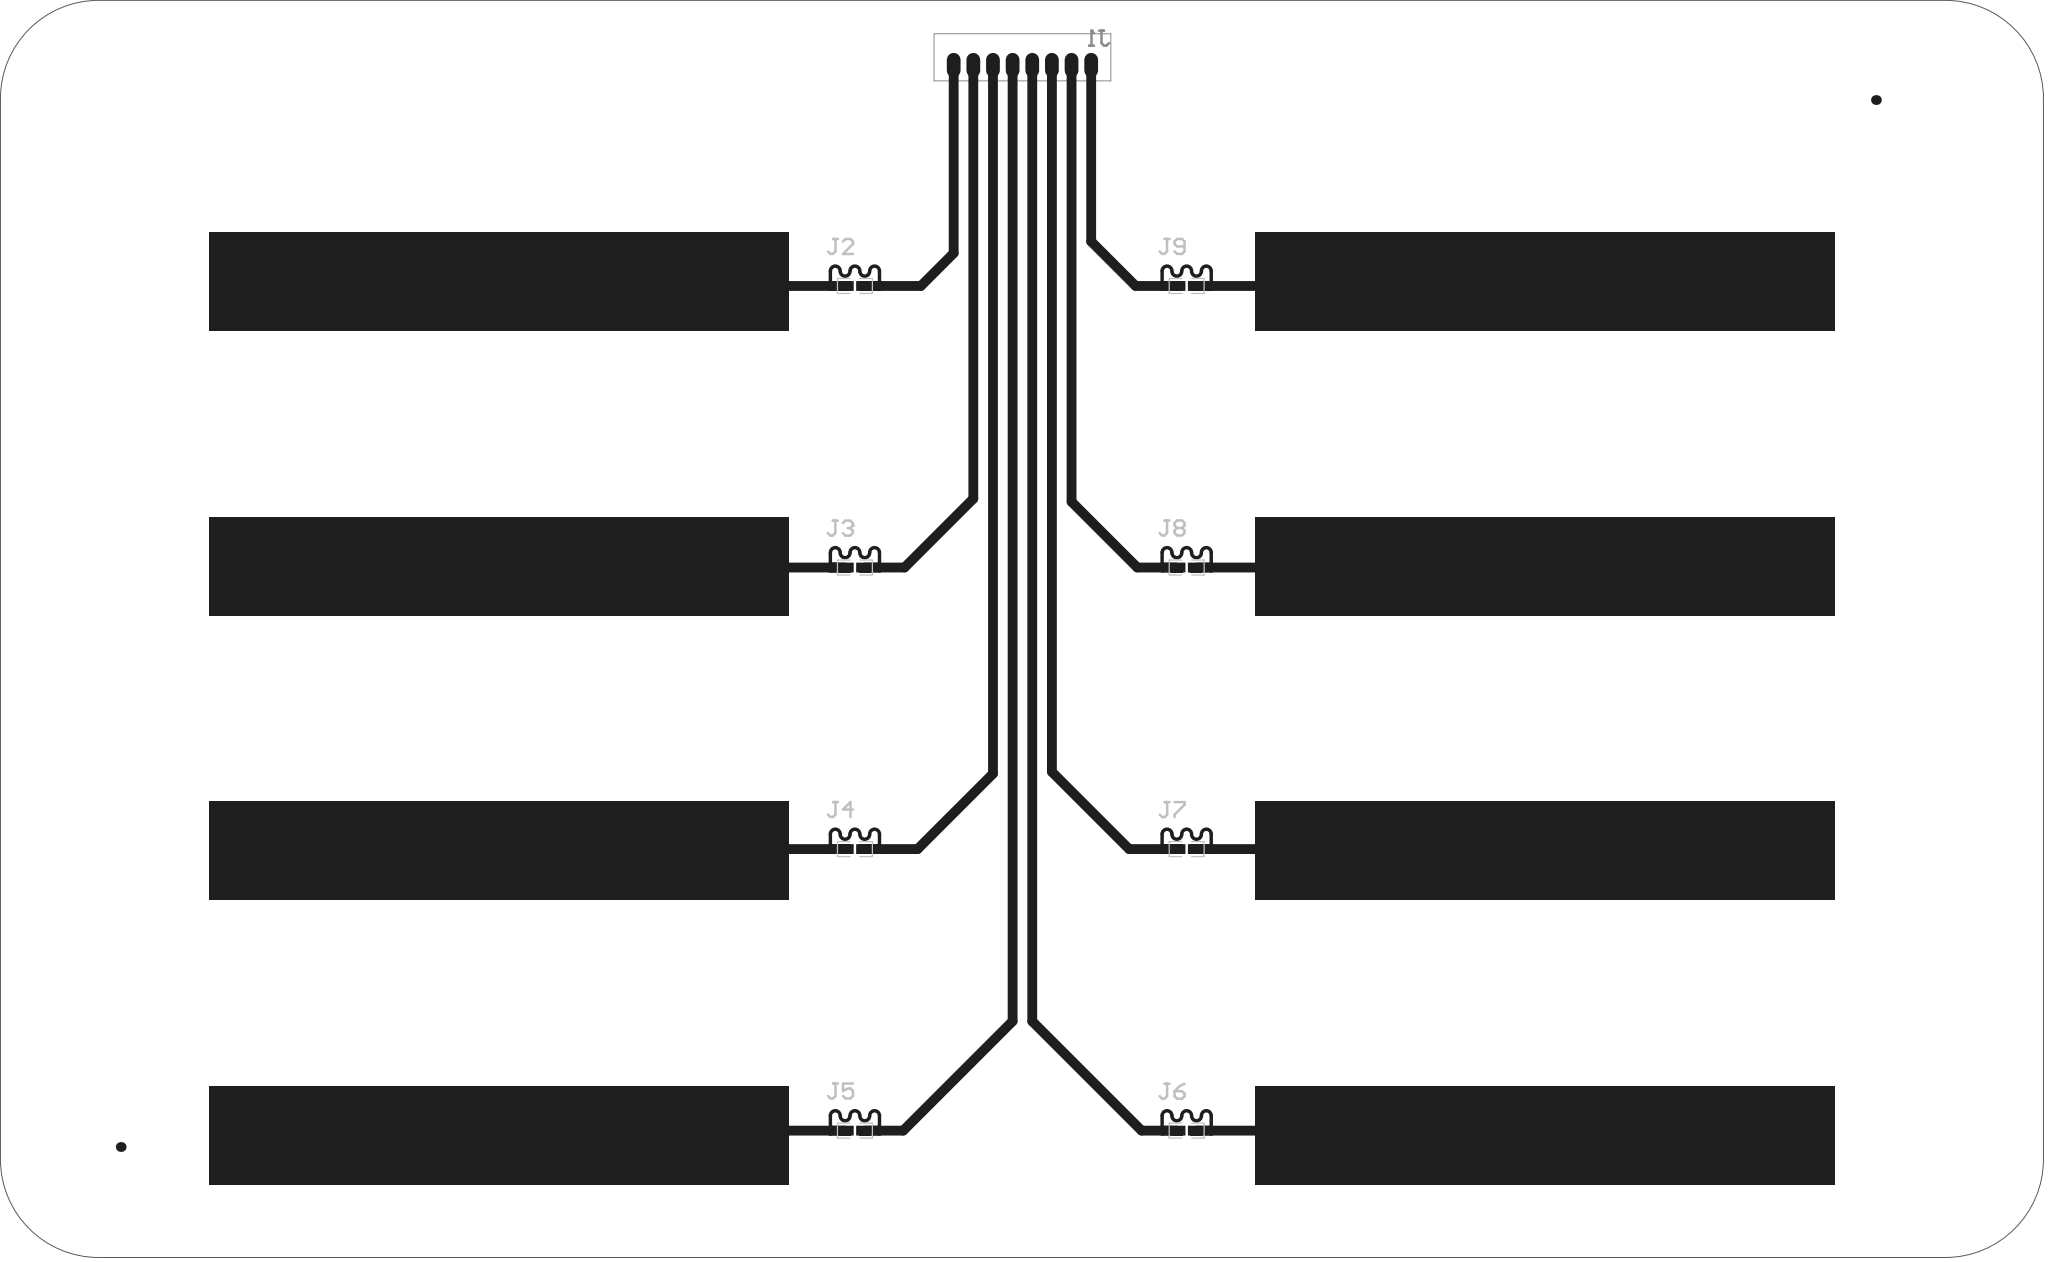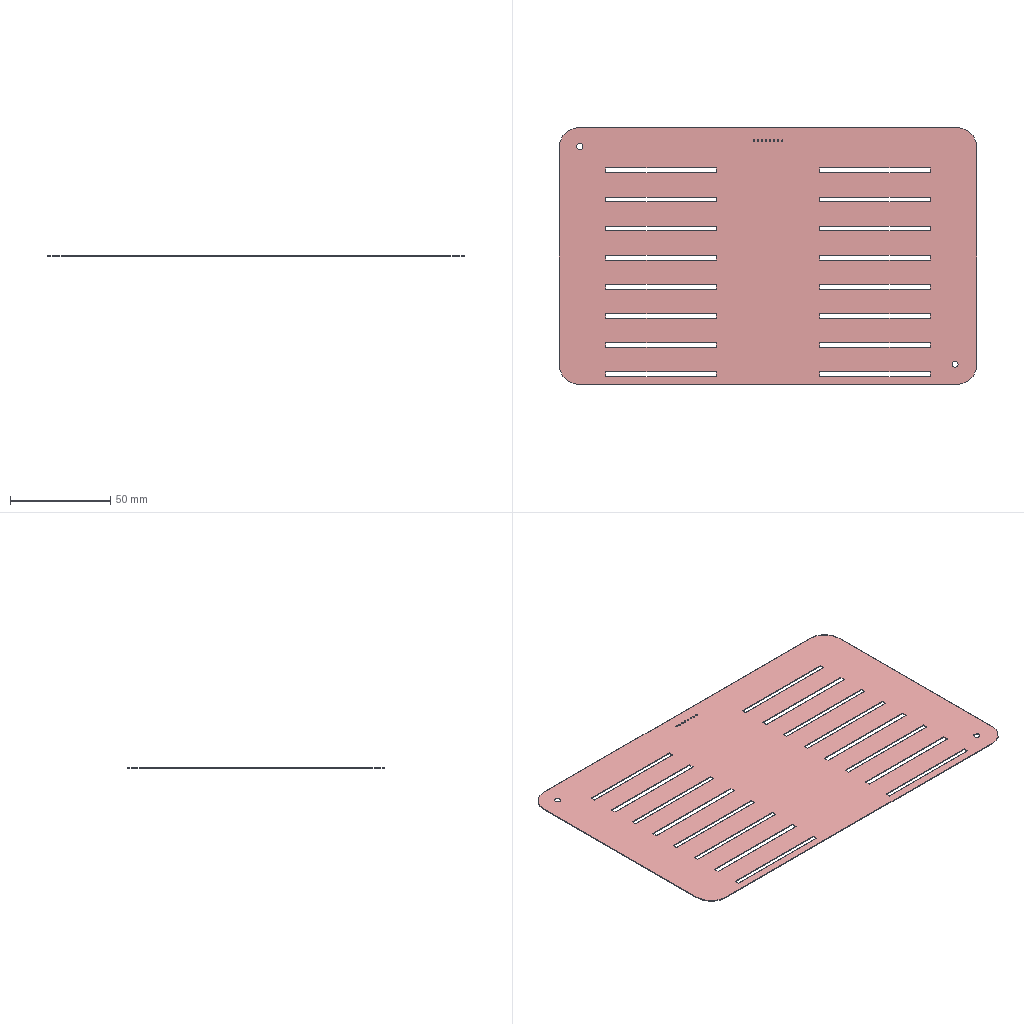Circuit board layout | Altium Designer | box 208 x 128 x 0.4 mm
Layer stack:
# Altium Designer layer stack of  (unit mm; dielectric type: 0 none, 1 core, 2 prepreg, 3 surface material)
index,name,kind,layer,copper_thickness_mm,dielectric_type,dielectric_thickness_mm,dielectric_material,dielectric_constant
0,Top Paste,other,,,,,,
1,Top Overlay,other,,,,,,
2,Top Solder,dielectric,,,3,0.0102,Solder Resist,3.5
3,Top Layer,copper,Top Layer,0.0356,,,,
4,Dielectric 1,dielectric,,,0,0.32,FR-4,4.8
5,Bottom Layer,copper,Bottom Layer,0.0356,,,,
6,Bottom Solder,dielectric,,,3,0.0102,Solder Resist,3.5
7,Bottom Overlay,other,,,,,,
8,Bottom Paste,other,,,,,,
# drill layer pairs: low layer,high layer
drill_pair,Top Layer,Bottom Layer
Part placement:
Designator,Comment,Layer,Footprint,Center-X(mm),Center-Y(mm),Rotation
B15,Pth,TopLayer,55*10*1MM,147.25,89.4,180
B13,Pth,TopLayer,55*10*1MM,147.25,60.4,180
B11,Pth,TopLayer,55*10*1MM,147.25,31.4,180
B9,Pth,TopLayer,55*10*1MM,147.25,2.4,180
B5,Pth,TopLayer,55*10*1MM,40.75,31.4,180
B3,Pth,TopLayer,55*10*1MM,40.75,60.4,180
B1,Pth,TopLayer,55*10*1MM,40.75,89.4,180
B7,Pth,TopLayer,55*10*1MM,40.75,2.4,180
J9,FPC,TopLayer,异形电阻,110.771,88.917,90
J3,FPC,TopLayer,异形电阻,76.996,60.251,90
J7,FPC,TopLayer,异形电阻,110.771,31.584,90
J5,FPC,TopLayer,异形电阻,76.996,2.917,90
J8,FPC,TopLayer,异形电阻,110.771,60.251,90
J6,FPC,TopLayer,异形电阻,110.771,2.917,90
J4,FPC,TopLayer,异形电阻,76.996,31.584,90
J2,FPC,TopLayer,异形电阻,76.996,88.917,90
J1,HX-2.0mm-8P THT connector with latch,BottomLayer,HX2.0-8P,94.05,111.4,0
Pad and via stacks:
# Altium Designer via and pad stacks of  (unit mm). Each distinct definition once, with the count of objects using it.
# via: kind,start_layer,end_layer,hole_mm,diameter_mm,mode(0 simple;1 top-mid-bottom;2 full stack),diameter_per_layer,count,example_net
# pad: kind,layer,hole_mm,hole_type(0 round;1 square;2 slot),plating,top_size,top_shape(1 round;2 rect;3 octagon;9 rounded rect),mid_size,bottom_size,mode,footprint,size_per_layer,count,example
pad,Top Layer,0,0,plated,1.4x2.5,1,1.4x2.5,1.4x2.5,0,HX2.0-8P,,8,J1.6
pad,Top Layer,0,2,plated,1x1,2,1x1,1x1,0,55*10*1MM,,8,B7.1
pad,Top Layer,0,0,plated,1.2x1,2,1.2x1,1.2x1,0,\u00D2\u00EC\u00D0\u00CE\u00B5\u00E7\u00D7\u00E8,,16,J3.2
pad,Top Layer,0,0,plated,1x1,1,1x1,1x1,0,,,2,3
pad,Multi-Layer,0.75,0,plated,0.75x0.75,1,0.75x0.75,0.75x0.75,0,HX2.0-8P,,8,J1.8
Design rules, without the lines most boards share:
# Altium Designer design rules of  (exported by Altium Designer, unit mm)
# columns: name | kind | enabled | priority | scope1 | scope2 | descriptor | typed fields (field=value)
NetAntennae | 56 | enabled | 1 | All | All | Net Antennae (Tolerance=0mm) (All) |
SilkToSilkClearance | 55 | enabled | 1 | All | All | Silk to Silk (Clearance=0mm) (All),(All) |
SilkToSolderMaskClearance | 54 | enabled | 1 | IsPad | All | Silk To Solder Mask (Clearance=0mm) (IsPad),(All) |
MinimumSolderMaskSliver | 53 | enabled | 1 | All | All | Minimum Solder Mask Sliver (Gap=0mm) (All),(All) |
HoleToHoleClearance | 52 | enabled | 1 | All | All | Hole To Hole Clearance (Gap=0mm) (All),(All) | gap=0
DiffPairsRouting | 51 | enabled | 1 | All | All | Differential Pairs Uncoupled Length using the Gap Constraints (Min=0.254mm) (Max=0.254mm) (Prefered=0.254mm)  and Width Constraints (Min=0.381mm) (Max=0.381mm) (Prefered=0.381mm) (All) |
HoleSize | 42 | enabled | 1 | All | All | Hole Size Constraint (Min=0.025mm) (Max=2.54mm) (All) |
Height | 50 | enabled | 1 | All | All | Height Constraint (Min=0mm) (Max=25.4mm) (Prefered=12.7mm) (All) | min_height=0 max_height=25.4
ComponentClearance | 24 | enabled | 1 | All | All | Component Clearance Constraint ( Horizontal Gap = 0mm, Vertical Gap = 0mm ) (All),(All)  | gap=0
SolderMaskExpansion | 13 | enabled | 1 | All | All | Solder Mask Expansion (Expansion =0.102mm) (All) | expansion=0.1016
PasteMaskExpansion | 14 | enabled | 1 | All | All | Paste Mask Expansion (Expansion =0mm) (All) | expansion=0
RoutingVias | 11 | enabled | 1 | All | All | Routing Via (MinHoleWidth=0.711mm) (MaxHoleWidth=0.711mm) (PreferredHoleWidth=0.711mm) (MinWidth=1.27mm) (MaxWidth=1.27mm) (PreferedWidth=1.27mm) (All) | via_min_hole=0.7112 via_max_hole=0.7112 via_preferred_diameter=1.27 via_preferred_hole=0.7112
RoutingCorners | 10 | enabled | 1 | All | All | Routing Corners (Style=45-Degree) (Min Setback=2.54mm) (Max Setback=2.54mm) (All) |
Width | 2 | enabled | 1 | All | All | Width Constraint (Min=0.254mm) (Max=2mm) (Preferred=0.254mm) (All) |
PolygonConnect | 20 | enabled | 1 | All | All | Polygon Connect Rule(Direct Connect )(Conductor Width=0.254mm) (Relief Angle=90 Angle) (Entries=4) (Air Gap Width=0.254mm) (All),(All) | connect_style(0=relief,1=direct,2=none)=1 relief_conductor_width=0.254 relief_entries=4
PlaneClearance | 12 | enabled | 1 | All | All | Power Plane Clearance (Clearance =0.508mm) (All) | clearance=0.508
PlaneConnect | 6 | enabled | 1 | All | All | Power Plane Connect Rule(Relief Connect )(Expansion=0.508mm) (Conductor Width=0.254mm) (Air Gap=0.254mm) (Entries=4) (All) | relief_conductor_width=0.254 relief_entries=4 relief_expansion=0.508
Clearance | 0 | enabled | 1 | All | All | Clearance Constraint (Gap=0.01mm) (All),(All) | gap=0.01
Classes set for this board:
# Altium Designer classes of  (member kind: 0 net, 1 component, 2 from-to, 3 pad, 4 layer, 5 differential pair, 6 design channel, 7 polygon, 8 structure, 9 xSignal)
# columns: class name | member kind | superclass | members
B-TRAN-MD27 V0 | 1 | no | J1; J2; J4; J6; J8; J5; J7; J3; J9; B7; B1; B3; B5; B9; B11; B13; B15;